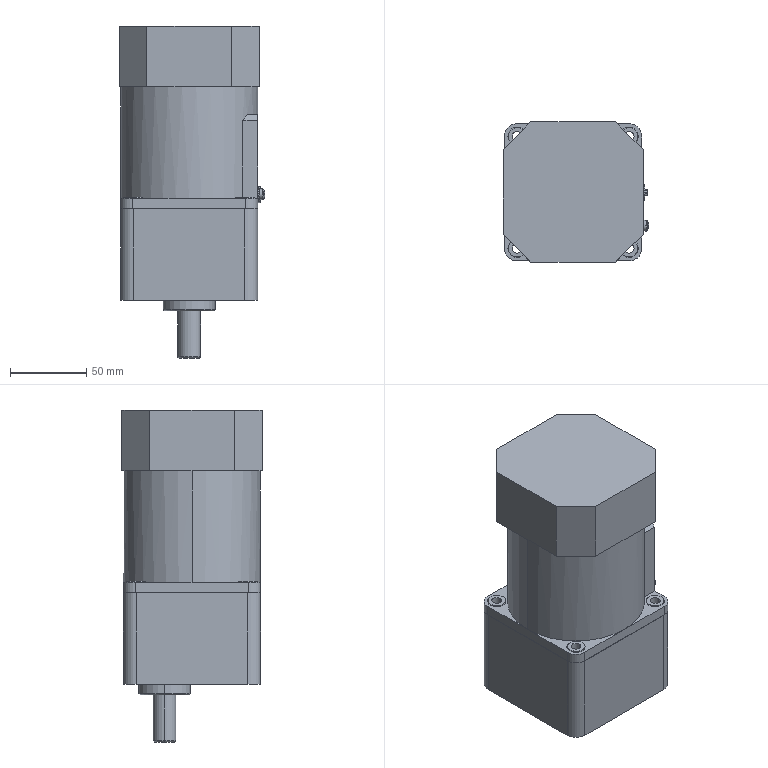Part | SolidWorks | features RefAxis 54, 3DProfileFeature 18, ICE 8, Revolution 5, LPattern 2, Extrusion 1, RevCut 1 | 1 solid | 124 faces | box 95.773 x 92 x 218 mm | volume 1327877 mm3 | plane 60 | cylinder 48 | torus 14 | sphere 2 | commonest cylinder face diameters 6.5 x8 12 x8 2 x6 14 x4 16 x4 16.66 x4